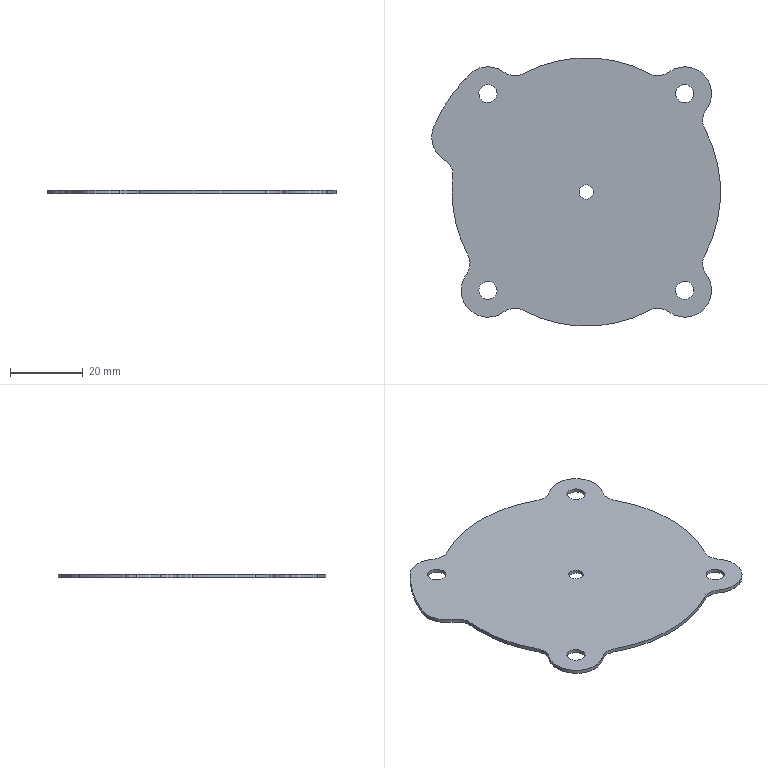Part | SolidWorks | features Cut 1, Extrusion 1 | 1 solid | 36 faces | box 79.627 x 74 x 1 mm | volume 4806 mm3 | cylinder 33 | plane 3 | commonest cylinder face diameters 10 x10 5 x8 14.784 x5 74 x5 4 x2 15 x2
STEP:
#1=CARTESIAN_POINT('',(2.,0.,1.));
#2=VERTEX_POINT('',#1);
#3=CARTESIAN_POINT('',(-2.,0.,1.));
#4=VERTEX_POINT('',#3);
#5=CARTESIAN_POINT('',(0.,0.,1.));
#6=DIRECTION('',(0.,0.,-1.));
#7=DIRECTION('',(-1.,0.,0.));
#8=AXIS2_PLACEMENT_3D('',#5,#6,#7);
#9=CIRCLE('',#8,2.);
#10=EDGE_CURVE('',#2,#4,#9,.T.);
#11=ORIENTED_EDGE('',*,*,#10,.F.);
#12=CARTESIAN_POINT('',(2.,0.,0.));
#13=VERTEX_POINT('',#12);
#14=CARTESIAN_POINT('',(2.,0.,1.));
#15=DIRECTION('',(0.,0.,-1.));
#16=VECTOR('',#15,1000.);
#17=LINE('',#14,#16);
#18=EDGE_CURVE('',#2,#13,#17,.T.);
#19=ORIENTED_EDGE('',*,*,#18,.T.);
#20=CARTESIAN_POINT('',(-2.,0.,0.));
#21=VERTEX_POINT('',#20);
#22=CARTESIAN_POINT('',(0.,0.,0.));
#23=DIRECTION('',(0.,0.,-1.));
#24=DIRECTION('',(-1.,0.,0.));
#25=AXIS2_PLACEMENT_3D('',#22,#23,#24);
#26=CIRCLE('',#25,2.);
#27=EDGE_CURVE('',#13,#21,#26,.T.);
#28=ORIENTED_EDGE('',*,*,#27,.T.);
#29=CARTESIAN_POINT('',(-2.,0.,1.));
#30=DIRECTION('',(0.,0.,-1.));
#31=VECTOR('',#30,1000.);
#32=LINE('',#29,#31);
#33=EDGE_CURVE('',#4,#21,#32,.T.);
#34=ORIENTED_EDGE('',*,*,#33,.F.);
#35=EDGE_LOOP('',(#11,#19,#28,#34));
#36=FACE_OUTER_BOUND('',#35,.T.);
#37=CARTESIAN_POINT('',(0.,0.,1.));
#38=DIRECTION('',(0.,0.,-1.));
#39=DIRECTION('',(-1.,0.,0.));
#40=AXIS2_PLACEMENT_3D('',#37,#38,#39);
#41=CYLINDRICAL_SURFACE('',#40,2.);
#42=ADVANCED_FACE('',(#36),#41,.F.);
#43=CARTESIAN_POINT('',(-29.633,27.133,1.));
#44=VERTEX_POINT('',#43);
#45=CARTESIAN_POINT('',(-24.633,27.133,1.));
#46=VERTEX_POINT('',#45);
#47=CARTESIAN_POINT('',(-29.633,27.133,1.));
#48=CARTESIAN_POINT('',(-29.633,26.098,1.));
#49=CARTESIAN_POINT('',(-28.901,25.366,1.));
#50=CARTESIAN_POINT('',(-28.169,24.633,1.));
#51=CARTESIAN_POINT('',(-27.133,24.633,1.));
#52=CARTESIAN_POINT('',(-26.098,24.633,1.));
#53=CARTESIAN_POINT('',(-25.366,25.366,1.));
#54=CARTESIAN_POINT('',(-24.633,26.098,1.));
#55=CARTESIAN_POINT('',(-24.633,27.133,1.));
#56=(BOUNDED_CURVE()B_SPLINE_CURVE(2,(#47,#48,#49,#50,#51,#52,#53,#54,#55),.UNSPECIFIED.,.F.,.T.)B_SPLINE_CURVE_WITH_KNOTS((3,2,2,2,3),(0.95,0.9583,0.9667,0.975,0.9833),.UNSPECIFIED.)CURVE()GEOMETRIC_REPRESENTATION_ITEM()RATIONAL_B_SPLINE_CURVE((1.,0.9239,1.,0.9239,1.,0.9239,1.,0.9239,1.))REPRESENTATION_ITEM(''));
#57=EDGE_CURVE('',#44,#46,#56,.T.);
#58=ORIENTED_EDGE('',*,*,#57,.T.);
#59=CARTESIAN_POINT('',(-24.633,27.133,0.));
#60=VERTEX_POINT('',#59);
#61=CARTESIAN_POINT('',(-24.633,27.133,1.));
#62=DIRECTION('',(0.,0.,-1.));
#63=VECTOR('',#62,1000.);
#64=LINE('',#61,#63);
#65=EDGE_CURVE('',#46,#60,#64,.T.);
#66=ORIENTED_EDGE('',*,*,#65,.T.);
#67=CARTESIAN_POINT('',(-29.633,27.133,0.));
#68=VERTEX_POINT('',#67);
#69=CARTESIAN_POINT('',(-29.633,27.133,0.));
#70=CARTESIAN_POINT('',(-29.633,26.098,0.));
#71=CARTESIAN_POINT('',(-28.901,25.366,0.));
#72=CARTESIAN_POINT('',(-28.169,24.633,0.));
#73=CARTESIAN_POINT('',(-27.133,24.633,0.));
#74=CARTESIAN_POINT('',(-26.098,24.633,0.));
#75=CARTESIAN_POINT('',(-25.366,25.366,0.));
#76=CARTESIAN_POINT('',(-24.633,26.098,0.));
#77=CARTESIAN_POINT('',(-24.633,27.133,0.));
#78=(BOUNDED_CURVE()B_SPLINE_CURVE(2,(#69,#70,#71,#72,#73,#74,#75,#76,#77),.UNSPECIFIED.,.F.,.F.)B_SPLINE_CURVE_WITH_KNOTS((3,2,2,2,3),(0.95,0.9583,0.9667,0.975,0.9833),.UNSPECIFIED.)CURVE()GEOMETRIC_REPRESENTATION_ITEM()RATIONAL_B_SPLINE_CURVE((1.,0.9239,1.,0.9239,1.,0.9239,1.,0.9239,1.))REPRESENTATION_ITEM(''));
#79=EDGE_CURVE('',#68,#60,#78,.T.);
#80=ORIENTED_EDGE('',*,*,#79,.F.);
#81=CARTESIAN_POINT('',(-29.633,27.133,1.));
#82=DIRECTION('',(0.,0.,-1.));
#83=VECTOR('',#82,1000.);
#84=LINE('',#81,#83);
#85=EDGE_CURVE('',#44,#68,#84,.T.);
#86=ORIENTED_EDGE('',*,*,#85,.F.);
#87=EDGE_LOOP('',(#58,#66,#80,#86));
#88=FACE_OUTER_BOUND('',#87,.T.);
#89=CARTESIAN_POINT('',(-27.133,27.133,1.));
#90=DIRECTION('',(0.,0.,-1.));
#91=DIRECTION('',(-1.,0.,0.));
#92=AXIS2_PLACEMENT_3D('',#89,#90,#91);
#93=CYLINDRICAL_SURFACE('',#92,2.5);
#94=ADVANCED_FACE('',(#88),#93,.F.);
#95=CARTESIAN_POINT('',(28.901,-28.901,1.));
#96=VERTEX_POINT('',#95);
#97=CARTESIAN_POINT('',(29.633,-27.133,1.));
#98=VERTEX_POINT('',#97);
#99=CARTESIAN_POINT('',(28.901,-28.901,1.));
#100=CARTESIAN_POINT('',(29.633,-28.169,1.));
#101=CARTESIAN_POINT('',(29.633,-27.133,1.));
#102=(BOUNDED_CURVE()B_SPLINE_CURVE(2,(#99,#100,#101),.UNSPECIFIED.,.F.,.F.)B_SPLINE_CURVE_WITH_KNOTS((3,3),(0.9417,0.95),.UNSPECIFIED.)CURVE()GEOMETRIC_REPRESENTATION_ITEM()RATIONAL_B_SPLINE_CURVE((1.,0.9239,1.))REPRESENTATION_ITEM(''));
#103=EDGE_CURVE('',#96,#98,#102,.T.);
#104=ORIENTED_EDGE('',*,*,#103,.T.);
#105=CARTESIAN_POINT('',(29.633,-27.133,0.));
#106=VERTEX_POINT('',#105);
#107=CARTESIAN_POINT('',(29.633,-27.133,1.));
#108=DIRECTION('',(0.,0.,-1.));
#109=VECTOR('',#108,1000.);
#110=LINE('',#107,#109);
#111=EDGE_CURVE('',#98,#106,#110,.T.);
#112=ORIENTED_EDGE('',*,*,#111,.T.);
#113=CARTESIAN_POINT('',(28.901,-28.901,0.));
#114=VERTEX_POINT('',#113);
#115=CARTESIAN_POINT('',(28.901,-28.901,0.));
#116=CARTESIAN_POINT('',(29.633,-28.169,0.));
#117=CARTESIAN_POINT('',(29.633,-27.133,0.));
#118=(BOUNDED_CURVE()B_SPLINE_CURVE(2,(#115,#116,#117),.UNSPECIFIED.,.F.,.T.)B_SPLINE_CURVE_WITH_KNOTS((3,3),(0.9417,0.95),.UNSPECIFIED.)CURVE()GEOMETRIC_REPRESENTATION_ITEM()RATIONAL_B_SPLINE_CURVE((1.,0.9239,1.))REPRESENTATION_ITEM(''));
#119=EDGE_CURVE('',#114,#106,#118,.T.);
#120=ORIENTED_EDGE('',*,*,#119,.F.);
#121=CARTESIAN_POINT('',(27.133,-29.633,0.));
#122=VERTEX_POINT('',#121);
#123=CARTESIAN_POINT('',(27.133,-27.133,0.));
#124=DIRECTION('',(0.,0.,1.));
#125=DIRECTION('',(1.,0.,0.));
#126=AXIS2_PLACEMENT_3D('',#123,#124,#125);
#127=CIRCLE('',#126,2.5);
#128=EDGE_CURVE('',#122,#114,#127,.T.);
#129=ORIENTED_EDGE('',*,*,#128,.F.);
#130=CARTESIAN_POINT('',(24.633,-27.133,0.));
#131=VERTEX_POINT('',#130);
#132=CARTESIAN_POINT('',(24.633,-27.133,0.));
#133=CARTESIAN_POINT('',(24.633,-28.169,0.));
#134=CARTESIAN_POINT('',(25.366,-28.901,0.));
#135=CARTESIAN_POINT('',(26.098,-29.633,0.));
#136=CARTESIAN_POINT('',(27.133,-29.633,0.));
#137=(BOUNDED_CURVE()B_SPLINE_CURVE(2,(#132,#133,#134,#135,#136),.UNSPECIFIED.,.F.,.T.)B_SPLINE_CURVE_WITH_KNOTS((3,2,3),(0.9833,0.9917,1.),.UNSPECIFIED.)CURVE()GEOMETRIC_REPRESENTATION_ITEM()RATIONAL_B_SPLINE_CURVE((1.,0.9239,1.,0.9239,1.))REPRESENTATION_ITEM(''));
#138=EDGE_CURVE('',#131,#122,#137,.T.);
#139=ORIENTED_EDGE('',*,*,#138,.F.);
#140=CARTESIAN_POINT('',(24.633,-27.133,1.));
#141=VERTEX_POINT('',#140);
#142=CARTESIAN_POINT('',(24.633,-27.133,1.));
#143=DIRECTION('',(0.,0.,-1.));
#144=VECTOR('',#143,1000.);
#145=LINE('',#142,#144);
#146=EDGE_CURVE('',#141,#131,#145,.T.);
#147=ORIENTED_EDGE('',*,*,#146,.F.);
#148=CARTESIAN_POINT('',(27.133,-29.633,1.));
#149=VERTEX_POINT('',#148);
#150=CARTESIAN_POINT('',(24.633,-27.133,1.));
#151=CARTESIAN_POINT('',(24.633,-28.169,1.));
#152=CARTESIAN_POINT('',(25.366,-28.901,1.));
#153=CARTESIAN_POINT('',(26.098,-29.633,1.));
#154=CARTESIAN_POINT('',(27.133,-29.633,1.));
#155=(BOUNDED_CURVE()B_SPLINE_CURVE(2,(#150,#151,#152,#153,#154),.UNSPECIFIED.,.F.,.F.)B_SPLINE_CURVE_WITH_KNOTS((3,2,3),(0.9833,0.9917,1.),.UNSPECIFIED.)CURVE()GEOMETRIC_REPRESENTATION_ITEM()RATIONAL_B_SPLINE_CURVE((1.,0.9239,1.,0.9239,1.))REPRESENTATION_ITEM(''));
#156=EDGE_CURVE('',#141,#149,#155,.T.);
#157=ORIENTED_EDGE('',*,*,#156,.T.);
#158=CARTESIAN_POINT('',(27.133,-27.133,1.));
#159=DIRECTION('',(0.,0.,1.));
#160=DIRECTION('',(1.,0.,0.));
#161=AXIS2_PLACEMENT_3D('',#158,#159,#160);
#162=CIRCLE('',#161,2.5);
#163=EDGE_CURVE('',#149,#96,#162,.T.);
#164=ORIENTED_EDGE('',*,*,#163,.T.);
#165=EDGE_LOOP('',(#104,#112,#120,#129,#139,#147,#157,#164));
#166=FACE_OUTER_BOUND('',#165,.T.);
#167=CARTESIAN_POINT('',(27.133,-27.133,1.));
#168=DIRECTION('',(0.,0.,-1.));
#169=DIRECTION('',(-1.,0.,0.));
#170=AXIS2_PLACEMENT_3D('',#167,#168,#169);
#171=CYLINDRICAL_SURFACE('',#170,2.5);
#172=ADVANCED_FACE('',(#166),#171,.F.);
#173=CARTESIAN_POINT('',(24.633,27.133,1.));
#174=VERTEX_POINT('',#173);
#175=CARTESIAN_POINT('',(29.633,27.133,1.));
#176=VERTEX_POINT('',#175);
#177=CARTESIAN_POINT('',(27.133,27.133,1.));
#178=DIRECTION('',(0.,0.,1.));
#179=DIRECTION('',(1.,0.,0.));
#180=AXIS2_PLACEMENT_3D('',#177,#178,#179);
#181=CIRCLE('',#180,2.5);
#182=EDGE_CURVE('',#174,#176,#181,.T.);
#183=ORIENTED_EDGE('',*,*,#182,.T.);
#184=CARTESIAN_POINT('',(29.633,27.133,0.));
#185=VERTEX_POINT('',#184);
#186=CARTESIAN_POINT('',(29.633,27.133,1.));
#187=DIRECTION('',(0.,0.,-1.));
#188=VECTOR('',#187,1000.);
#189=LINE('',#186,#188);
#190=EDGE_CURVE('',#176,#185,#189,.T.);
#191=ORIENTED_EDGE('',*,*,#190,.T.);
#192=CARTESIAN_POINT('',(24.633,27.133,0.));
#193=VERTEX_POINT('',#192);
#194=CARTESIAN_POINT('',(27.133,27.133,0.));
#195=DIRECTION('',(0.,0.,1.));
#196=DIRECTION('',(1.,0.,0.));
#197=AXIS2_PLACEMENT_3D('',#194,#195,#196);
#198=CIRCLE('',#197,2.5);
#199=EDGE_CURVE('',#193,#185,#198,.T.);
#200=ORIENTED_EDGE('',*,*,#199,.F.);
#201=CARTESIAN_POINT('',(24.633,27.133,1.));
#202=DIRECTION('',(0.,0.,-1.));
#203=VECTOR('',#202,1000.);
#204=LINE('',#201,#203);
#205=EDGE_CURVE('',#174,#193,#204,.T.);
#206=ORIENTED_EDGE('',*,*,#205,.F.);
#207=EDGE_LOOP('',(#183,#191,#200,#206));
#208=FACE_OUTER_BOUND('',#207,.T.);
#209=CARTESIAN_POINT('',(27.133,27.133,1.));
#210=DIRECTION('',(0.,0.,-1.));
#211=DIRECTION('',(-1.,0.,0.));
#212=AXIS2_PLACEMENT_3D('',#209,#210,#211);
#213=CYLINDRICAL_SURFACE('',#212,2.5);
#214=ADVANCED_FACE('',(#208),#213,.F.);
#215=CARTESIAN_POINT('',(-28.901,-28.901,1.));
#216=VERTEX_POINT('',#215);
#217=CARTESIAN_POINT('',(-24.633,-27.133,1.));
#218=VERTEX_POINT('',#217);
#219=CARTESIAN_POINT('',(-28.901,-28.901,1.));
#220=CARTESIAN_POINT('',(-28.169,-29.633,1.));
#221=CARTESIAN_POINT('',(-27.133,-29.633,1.));
#222=CARTESIAN_POINT('',(-26.098,-29.633,1.));
#223=CARTESIAN_POINT('',(-25.366,-28.901,1.));
#224=CARTESIAN_POINT('',(-24.633,-28.169,1.));
#225=CARTESIAN_POINT('',(-24.633,-27.133,1.));
#226=(BOUNDED_CURVE()B_SPLINE_CURVE(2,(#219,#220,#221,#222,#223,#224,#225),.UNSPECIFIED.,.F.,.T.)B_SPLINE_CURVE_WITH_KNOTS((3,2,2,3),(0.9417,0.95,0.9583,0.9667),.UNSPECIFIED.)CURVE()GEOMETRIC_REPRESENTATION_ITEM()RATIONAL_B_SPLINE_CURVE((1.,0.9239,1.,0.9239,1.,0.9239,1.))REPRESENTATION_ITEM(''));
#227=EDGE_CURVE('',#216,#218,#226,.T.);
#228=ORIENTED_EDGE('',*,*,#227,.T.);
#229=CARTESIAN_POINT('',(-24.633,-27.133,0.));
#230=VERTEX_POINT('',#229);
#231=CARTESIAN_POINT('',(-24.633,-27.133,1.));
#232=DIRECTION('',(0.,0.,-1.));
#233=VECTOR('',#232,1000.);
#234=LINE('',#231,#233);
#235=EDGE_CURVE('',#218,#230,#234,.T.);
#236=ORIENTED_EDGE('',*,*,#235,.T.);
#237=CARTESIAN_POINT('',(-28.901,-28.901,0.));
#238=VERTEX_POINT('',#237);
#239=CARTESIAN_POINT('',(-28.901,-28.901,0.));
#240=CARTESIAN_POINT('',(-28.169,-29.633,0.));
#241=CARTESIAN_POINT('',(-27.133,-29.633,0.));
#242=CARTESIAN_POINT('',(-26.098,-29.633,0.));
#243=CARTESIAN_POINT('',(-25.366,-28.901,0.));
#244=CARTESIAN_POINT('',(-24.633,-28.169,0.));
#245=CARTESIAN_POINT('',(-24.633,-27.133,0.));
#246=(BOUNDED_CURVE()B_SPLINE_CURVE(2,(#239,#240,#241,#242,#243,#244,#245),.UNSPECIFIED.,.F.,.T.)B_SPLINE_CURVE_WITH_KNOTS((3,2,2,3),(0.9417,0.95,0.9583,0.9667),.UNSPECIFIED.)CURVE()GEOMETRIC_REPRESENTATION_ITEM()RATIONAL_B_SPLINE_CURVE((1.,0.9239,1.,0.9239,1.,0.9239,1.))REPRESENTATION_ITEM(''));
#247=EDGE_CURVE('',#238,#230,#246,.T.);
#248=ORIENTED_EDGE('',*,*,#247,.F.);
#249=CARTESIAN_POINT('',(-29.633,-27.133,0.));
#250=VERTEX_POINT('',#249);
#251=CARTESIAN_POINT('',(-27.133,-27.133,0.));
#252=DIRECTION('',(0.,0.,1.));
#253=DIRECTION('',(1.,0.,0.));
#254=AXIS2_PLACEMENT_3D('',#251,#252,#253);
#255=CIRCLE('',#254,2.5);
#256=EDGE_CURVE('',#250,#238,#255,.T.);
#257=ORIENTED_EDGE('',*,*,#256,.F.);
#258=CARTESIAN_POINT('',(-29.633,-27.133,1.));
#259=VERTEX_POINT('',#258);
#260=CARTESIAN_POINT('',(-29.633,-27.133,1.));
#261=DIRECTION('',(0.,0.,-1.));
#262=VECTOR('',#261,1000.);
#263=LINE('',#260,#262);
#264=EDGE_CURVE('',#259,#250,#263,.T.);
#265=ORIENTED_EDGE('',*,*,#264,.F.);
#266=CARTESIAN_POINT('',(-27.133,-27.133,1.));
#267=DIRECTION('',(0.,0.,1.));
#268=DIRECTION('',(1.,0.,0.));
#269=AXIS2_PLACEMENT_3D('',#266,#267,#268);
#270=CIRCLE('',#269,2.5);
#271=EDGE_CURVE('',#259,#216,#270,.T.);
#272=ORIENTED_EDGE('',*,*,#271,.T.);
#273=EDGE_LOOP('',(#228,#236,#248,#257,#265,#272));
#274=FACE_OUTER_BOUND('',#273,.T.);
#275=CARTESIAN_POINT('',(-27.133,-27.133,1.));
#276=DIRECTION('',(0.,0.,-1.));
#277=DIRECTION('',(-1.,0.,0.));
#278=AXIS2_PLACEMENT_3D('',#275,#276,#277);
#279=CYLINDRICAL_SURFACE('',#278,2.5);
#280=ADVANCED_FACE('',(#274),#279,.F.);
#281=CARTESIAN_POINT('',(32.075,19.735,1.));
#282=VERTEX_POINT('',#281);
#283=CARTESIAN_POINT('',(33.064,22.72,1.));
#284=VERTEX_POINT('',#283);
#285=CARTESIAN_POINT('',(37.075,19.735,1.));
#286=DIRECTION('',(0.,0.,-1.));
#287=DIRECTION('',(1.,0.,0.));
#288=AXIS2_PLACEMENT_3D('',#285,#286,#287);
#289=CIRCLE('',#288,5.);
#290=EDGE_CURVE('',#282,#284,#289,.T.);
#291=ORIENTED_EDGE('',*,*,#290,.F.);
#292=CARTESIAN_POINT('',(32.075,19.735,0.));
#293=VERTEX_POINT('',#292);
#294=CARTESIAN_POINT('',(32.075,19.735,1.));
#295=DIRECTION('',(0.,0.,-1.));
#296=VECTOR('',#295,1000.);
#297=LINE('',#294,#296);
#298=EDGE_CURVE('',#282,#293,#297,.T.);
#299=ORIENTED_EDGE('',*,*,#298,.T.);
#300=CARTESIAN_POINT('',(33.064,22.72,0.));
#301=VERTEX_POINT('',#300);
#302=CARTESIAN_POINT('',(37.075,19.735,0.));
#303=DIRECTION('',(0.,0.,-1.));
#304=DIRECTION('',(1.,0.,0.));
#305=AXIS2_PLACEMENT_3D('',#302,#303,#304);
#306=CIRCLE('',#305,5.);
#307=EDGE_CURVE('',#293,#301,#306,.T.);
#308=ORIENTED_EDGE('',*,*,#307,.T.);
#309=CARTESIAN_POINT('',(33.064,22.72,1.));
#310=DIRECTION('',(0.,0.,-1.));
#311=VECTOR('',#310,1000.);
#312=LINE('',#309,#311);
#313=EDGE_CURVE('',#284,#301,#312,.T.);
#314=ORIENTED_EDGE('',*,*,#313,.F.);
#315=EDGE_LOOP('',(#291,#299,#308,#314));
#316=FACE_OUTER_BOUND('',#315,.T.);
#317=CARTESIAN_POINT('',(37.075,19.735,1.));
#318=DIRECTION('',(0.,0.,-1.));
#319=DIRECTION('',(-1.,0.,0.));
#320=AXIS2_PLACEMENT_3D('',#317,#318,#319);
#321=CYLINDRICAL_SURFACE('',#320,5.);
#322=ADVANCED_FACE('',(#316),#321,.F.);
#323=CARTESIAN_POINT('',(32.075,-19.735,1.));
#324=VERTEX_POINT('',#323);
#325=CARTESIAN_POINT('',(32.661,-17.386,1.));
#326=VERTEX_POINT('',#325);
#327=CARTESIAN_POINT('',(37.075,-19.735,1.));
#328=DIRECTION('',(0.,0.,-1.));
#329=DIRECTION('',(1.,0.,0.));
#330=AXIS2_PLACEMENT_3D('',#327,#328,#329);
#331=CIRCLE('',#330,5.);
#332=EDGE_CURVE('',#324,#326,#331,.T.);
#333=ORIENTED_EDGE('',*,*,#332,.F.);
#334=CARTESIAN_POINT('',(32.075,-19.735,0.));
#335=VERTEX_POINT('',#334);
#336=CARTESIAN_POINT('',(32.075,-19.735,1.));
#337=DIRECTION('',(0.,0.,-1.));
#338=VECTOR('',#337,1000.);
#339=LINE('',#336,#338);
#340=EDGE_CURVE('',#324,#335,#339,.T.);
#341=ORIENTED_EDGE('',*,*,#340,.T.);
#342=CARTESIAN_POINT('',(32.661,-17.386,0.));
#343=VERTEX_POINT('',#342);
#344=CARTESIAN_POINT('',(37.075,-19.735,0.));
#345=DIRECTION('',(0.,0.,-1.));
#346=DIRECTION('',(1.,0.,0.));
#347=AXIS2_PLACEMENT_3D('',#344,#345,#346);
#348=CIRCLE('',#347,5.);
#349=EDGE_CURVE('',#335,#343,#348,.T.);
#350=ORIENTED_EDGE('',*,*,#349,.T.);
#351=CARTESIAN_POINT('',(32.661,-17.386,1.));
#352=DIRECTION('',(0.,0.,-1.));
#353=VECTOR('',#352,1000.);
#354=LINE('',#351,#353);
#355=EDGE_CURVE('',#326,#343,#354,.T.);
#356=ORIENTED_EDGE('',*,*,#355,.F.);
#357=EDGE_LOOP('',(#333,#341,#350,#356));
#358=FACE_OUTER_BOUND('',#357,.T.);
#359=CARTESIAN_POINT('',(37.075,-19.735,1.));
#360=DIRECTION('',(0.,0.,-1.));
#361=DIRECTION('',(-1.,0.,0.));
#362=AXIS2_PLACEMENT_3D('',#359,#360,#361);
#363=CYLINDRICAL_SURFACE('',#362,5.);
#364=ADVANCED_FACE('',(#358),#363,.F.);
#365=CARTESIAN_POINT('',(-34.526,-27.133,1.));
#366=VERTEX_POINT('',#365);
#367=CARTESIAN_POINT('',(-22.72,-33.064,1.));
#368=VERTEX_POINT('',#367);
#369=CARTESIAN_POINT('',(-27.133,-27.133,1.));
#370=DIRECTION('',(0.,0.,1.));
#371=DIRECTION('',(1.,0.,0.));
#372=AXIS2_PLACEMENT_3D('',#369,#370,#371);
#373=CIRCLE('',#372,7.392);
#374=EDGE_CURVE('',#366,#368,#373,.T.);
#375=ORIENTED_EDGE('',*,*,#374,.F.);
#376=CARTESIAN_POINT('',(-34.526,-27.133,0.));
#377=VERTEX_POINT('',#376);
#378=CARTESIAN_POINT('',(-34.526,-27.133,1.));
#379=DIRECTION('',(0.,0.,-1.));
#380=VECTOR('',#379,1000.);
#381=LINE('',#378,#380);
#382=EDGE_CURVE('',#366,#377,#381,.T.);
#383=ORIENTED_EDGE('',*,*,#382,.T.);
#384=CARTESIAN_POINT('',(-22.72,-33.064,0.));
#385=VERTEX_POINT('',#384);
#386=CARTESIAN_POINT('',(-27.133,-27.133,0.));
#387=DIRECTION('',(0.,0.,1.));
#388=DIRECTION('',(1.,0.,0.));
#389=AXIS2_PLACEMENT_3D('',#386,#387,#388);
#390=CIRCLE('',#389,7.392);
#391=EDGE_CURVE('',#377,#385,#390,.T.);
#392=ORIENTED_EDGE('',*,*,#391,.T.);
#393=CARTESIAN_POINT('',(-22.72,-33.064,1.));
#394=DIRECTION('',(0.,0.,-1.));
#395=VECTOR('',#394,1000.);
#396=LINE('',#393,#395);
#397=EDGE_CURVE('',#368,#385,#396,.T.);
#398=ORIENTED_EDGE('',*,*,#397,.F.);
#399=EDGE_LOOP('',(#375,#383,#392,#398));
#400=FACE_OUTER_BOUND('',#399,.T.);
#401=CARTESIAN_POINT('',(-27.133,-27.133,1.));
#402=DIRECTION('',(0.,0.,-1.));
#403=DIRECTION('',(-1.,0.,0.));
#404=AXIS2_PLACEMENT_3D('',#401,#402,#403);
#405=CYLINDRICAL_SURFACE('',#404,7.392);
#406=ADVANCED_FACE('',(#400),#405,.T.);
#407=CARTESIAN_POINT('',(-37.,0.,1.));
#408=VERTEX_POINT('',#407);
#409=CARTESIAN_POINT('',(-32.661,-17.386,1.));
#410=VERTEX_POINT('',#409);
#411=CARTESIAN_POINT('',(0.,0.,1.));
#412=DIRECTION('',(0.,0.,1.));
#413=DIRECTION('',(1.,0.,0.));
#414=AXIS2_PLACEMENT_3D('',#411,#412,#413);
#415=CIRCLE('',#414,37.);
#416=EDGE_CURVE('',#408,#410,#415,.T.);
#417=ORIENTED_EDGE('',*,*,#416,.F.);
#418=CARTESIAN_POINT('',(-37.,0.,0.));
#419=VERTEX_POINT('',#418);
#420=CARTESIAN_POINT('',(-37.,0.,1.));
#421=DIRECTION('',(0.,0.,-1.));
#422=VECTOR('',#421,1000.);
#423=LINE('',#420,#422);
#424=EDGE_CURVE('',#408,#419,#423,.T.);
#425=ORIENTED_EDGE('',*,*,#424,.T.);
#426=CARTESIAN_POINT('',(-32.661,-17.386,0.));
#427=VERTEX_POINT('',#426);
#428=CARTESIAN_POINT('',(0.,0.,0.));
#429=DIRECTION('',(0.,0.,1.));
#430=DIRECTION('',(1.,0.,0.));
#431=AXIS2_PLACEMENT_3D('',#428,#429,#430);
#432=CIRCLE('',#431,37.);
#433=EDGE_CURVE('',#419,#427,#432,.T.);
#434=ORIENTED_EDGE('',*,*,#433,.T.);
#435=CARTESIAN_POINT('',(-32.661,-17.386,1.));
#436=DIRECTION('',(0.,0.,-1.));
#437=VECTOR('',#436,1000.);
#438=LINE('',#435,#437);
#439=EDGE_CURVE('',#410,#427,#438,.T.);
#440=ORIENTED_EDGE('',*,*,#439,.F.);
#441=EDGE_LOOP('',(#417,#425,#434,#440));
#442=FACE_OUTER_BOUND('',#441,.T.);
#443=CARTESIAN_POINT('',(0.,0.,1.));
#444=DIRECTION('',(0.,0.,-1.));
#445=DIRECTION('',(-1.,0.,0.));
#446=AXIS2_PLACEMENT_3D('',#443,#444,#445);
#447=CYLINDRICAL_SURFACE('',#446,37.);
#448=ADVANCED_FACE('',(#442),#447,.T.);
#449=CARTESIAN_POINT('',(-42.627,15.175,1.));
#450=VERTEX_POINT('',#449);
#451=CARTESIAN_POINT('',(-39.101,8.815,1.));
#452=VERTEX_POINT('',#451);
#453=CARTESIAN_POINT('',(-35.127,15.175,1.));
#454=DIRECTION('',(0.,0.,1.));
#455=DIRECTION('',(1.,0.,0.));
#456=AXIS2_PLACEMENT_3D('',#453,#454,#455);
#457=CIRCLE('',#456,7.5);
#458=EDGE_CURVE('',#450,#452,#457,.T.);
#459=ORIENTED_EDGE('',*,*,#458,.F.);
#460=CARTESIAN_POINT('',(-42.627,15.175,0.));
#461=VERTEX_POINT('',#460);
#462=CARTESIAN_POINT('',(-42.627,15.175,1.));
#463=DIRECTION('',(0.,0.,-1.));
#464=VECTOR('',#463,1000.);
#465=LINE('',#462,#464);
#466=EDGE_CURVE('',#450,#461,#465,.T.);
#467=ORIENTED_EDGE('',*,*,#466,.T.);
#468=CARTESIAN_POINT('',(-39.101,8.815,0.));
#469=VERTEX_POINT('',#468);
#470=CARTESIAN_POINT('',(-35.127,15.175,0.));
#471=DIRECTION('',(0.,0.,1.));
#472=DIRECTION('',(1.,0.,0.));
#473=AXIS2_PLACEMENT_3D('',#470,#471,#472);
#474=CIRCLE('',#473,7.5);
#475=EDGE_CURVE('',#461,#469,#474,.T.);
#476=ORIENTED_EDGE('',*,*,#475,.T.);
#477=CARTESIAN_POINT('',(-39.101,8.815,1.));
#478=DIRECTION('',(0.,0.,-1.));
#479=VECTOR('',#478,1000.);
#480=LINE('',#477,#479);
#481=EDGE_CURVE('',#452,#469,#480,.T.);
#482=ORIENTED_EDGE('',*,*,#481,.F.);
#483=EDGE_LOOP('',(#459,#467,#476,#482));
#484=FACE_OUTER_BOUND('',#483,.T.);
#485=CARTESIAN_POINT('',(-35.127,15.175,1.));
#486=DIRECTION('',(0.,0.,-1.));
#487=DIRECTION('',(-1.,0.,0.));
#488=AXIS2_PLACEMENT_3D('',#485,#486,#487);
#489=CYLINDRICAL_SURFACE('',#488,7.5);
#490=ADVANCED_FACE('',(#484),#489,.T.);
#491=CARTESIAN_POINT('',(0.,0.,1.));
#492=DIRECTION('',(0.,0.,-1.));
#493=DIRECTION('',(-1.,0.,0.));
#494=AXIS2_PLACEMENT_3D('',#491,#492,#493);
#495=CIRCLE('',#494,2.);
#496=EDGE_CURVE('',#4,#2,#495,.T.);
#497=ORIENTED_EDGE('',*,*,#496,.T.);
#498=ORIENTED_EDGE('',*,*,#10,.T.);
#499=EDGE_LOOP('',(#497,#498));
#500=FACE_BOUND('',#499,.T.);
#501=ORIENTED_EDGE('',*,*,#227,.F.);
#502=ORIENTED_EDGE('',*,*,#271,.F.);
#503=CARTESIAN_POINT('',(-24.633,-27.133,1.));
#504=CARTESIAN_POINT('',(-24.633,-26.098,1.));
#505=CARTESIAN_POINT('',(-25.366,-25.366,1.));
#506=CARTESIAN_POINT('',(-26.098,-24.633,1.));
#507=CARTESIAN_POINT('',(-27.133,-24.633,1.));
#508=CARTESIAN_POINT('',(-28.169,-24.633,1.));
#509=CARTESIAN_POINT('',(-28.901,-25.366,1.));
#510=CARTESIAN_POINT('',(-29.633,-26.098,1.));
#511=CARTESIAN_POINT('',(-29.633,-27.133,1.));
#512=(BOUNDED_CURVE()B_SPLINE_CURVE(2,(#503,#504,#505,#506,#507,#508,#509,#510,#511),.UNSPECIFIED.,.F.,.F.)B_SPLINE_CURVE_WITH_KNOTS((3,2,2,2,3),(0.9667,0.975,0.9833,0.9917,1.),.UNSPECIFIED.)CURVE()GEOMETRIC_REPRESENTATION_ITEM()RATIONAL_B_SPLINE_CURVE((1.,0.9239,1.,0.9239,1.,0.9239,1.,0.9239,1.))REPRESENTATION_ITEM(''));
#513=EDGE_CURVE('',#218,#259,#512,.T.);
#514=ORIENTED_EDGE('',*,*,#513,.F.);
#515=EDGE_LOOP('',(#501,#502,#514));
#516=FACE_BOUND('',#515,.T.);
#517=CARTESIAN_POINT('',(-33.455,31.228,1.));
#518=VERTEX_POINT('',#517);
#519=CARTESIAN_POINT('',(-42.012,18.15,1.));
#520=VERTEX_POINT('',#519);
#521=CARTESIAN_POINT('',(0.,0.,1.));
#522=DIRECTION('',(0.,0.,1.));
#523=DIRECTION('',(1.,0.,0.));
#524=AXIS2_PLACEMENT_3D('',#521,#522,#523);
#525=CIRCLE('',#524,45.765);
#526=EDGE_CURVE('',#518,#520,#525,.T.);
#527=ORIENTED_EDGE('',*,*,#526,.T.);
#528=CARTESIAN_POINT('',(-35.127,15.175,1.));
#529=DIRECTION('',(0.,0.,1.));
#530=DIRECTION('',(1.,0.,0.));
#531=AXIS2_PLACEMENT_3D('',#528,#529,#530);
#532=CIRCLE('',#531,7.5);
#533=EDGE_CURVE('',#520,#450,#532,.T.);
#534=ORIENTED_EDGE('',*,*,#533,.T.);
#535=ORIENTED_EDGE('',*,*,#458,.T.);
#536=CARTESIAN_POINT('',(-36.78,4.03,1.));
#537=VERTEX_POINT('',#536);
#538=CARTESIAN_POINT('',(-41.75,4.574,1.));
#539=DIRECTION('',(0.,0.,-1.));
#540=DIRECTION('',(1.,0.,0.));
#541=AXIS2_PLACEMENT_3D('',#538,#539,#540);
#542=CIRCLE('',#541,5.);
#543=EDGE_CURVE('',#452,#537,#542,.T.);
#544=ORIENTED_EDGE('',*,*,#543,.T.);
#545=CARTESIAN_POINT('',(0.,0.,1.));
#546=DIRECTION('',(0.,0.,1.));
#547=DIRECTION('',(1.,0.,0.));
#548=AXIS2_PLACEMENT_3D('',#545,#546,#547);
#549=CIRCLE('',#548,37.);
#550=EDGE_CURVE('',#537,#408,#549,.T.);
#551=ORIENTED_EDGE('',*,*,#550,.T.);
#552=ORIENTED_EDGE('',*,*,#416,.T.);
#553=CARTESIAN_POINT('',(-33.064,-22.72,1.));
#554=VERTEX_POINT('',#553);
#555=CARTESIAN_POINT('',(-37.075,-19.735,1.));
#556=DIRECTION('',(0.,0.,-1.));
#557=DIRECTION('',(1.,0.,0.));
#558=AXIS2_PLACEMENT_3D('',#555,#556,#557);
#559=CIRCLE('',#558,5.);
#560=EDGE_CURVE('',#410,#554,#559,.T.);
#561=ORIENTED_EDGE('',*,*,#560,.T.);
#562=CARTESIAN_POINT('',(-27.133,-27.133,1.));
#563=DIRECTION('',(0.,0.,1.));
#564=DIRECTION('',(1.,0.,0.));
#565=AXIS2_PLACEMENT_3D('',#562,#563,#564);
#566=CIRCLE('',#565,7.392);
#567=EDGE_CURVE('',#554,#366,#566,.T.);
#568=ORIENTED_EDGE('',*,*,#567,.T.);
#569=ORIENTED_EDGE('',*,*,#374,.T.);
#570=CARTESIAN_POINT('',(-17.386,-32.661,1.));
#571=VERTEX_POINT('',#570);
#572=CARTESIAN_POINT('',(-19.735,-37.075,1.));
#573=DIRECTION('',(0.,0.,-1.));
#574=DIRECTION('',(1.,0.,0.));
#575=AXIS2_PLACEMENT_3D('',#572,#573,#574);
#576=CIRCLE('',#575,5.);
#577=EDGE_CURVE('',#368,#571,#576,.T.);
#578=ORIENTED_EDGE('',*,*,#577,.T.);
#579=CARTESIAN_POINT('',(17.386,-32.661,1.));
#580=VERTEX_POINT('',#579);
#581=CARTESIAN_POINT('',(0.,0.,1.));
#582=DIRECTION('',(0.,0.,1.));
#583=DIRECTION('',(1.,0.,0.));
#584=AXIS2_PLACEMENT_3D('',#581,#582,#583);
#585=CIRCLE('',#584,37.);
#586=EDGE_CURVE('',#571,#580,#585,.T.);
#587=ORIENTED_EDGE('',*,*,#586,.T.);
#588=CARTESIAN_POINT('',(22.72,-33.064,1.));
#589=VERTEX_POINT('',#588);
#590=CARTESIAN_POINT('',(19.735,-37.075,1.));
#591=DIRECTION('',(0.,0.,-1.));
#592=DIRECTION('',(1.,0.,0.));
#593=AXIS2_PLACEMENT_3D('',#590,#591,#592);
#594=CIRCLE('',#593,5.);
#595=EDGE_CURVE('',#580,#589,#594,.T.);
#596=ORIENTED_EDGE('',*,*,#595,.T.);
#597=CARTESIAN_POINT('',(33.064,-22.72,1.));
#598=VERTEX_POINT('',#597);
#599=CARTESIAN_POINT('',(27.133,-27.133,1.));
#600=DIRECTION('',(0.,0.,1.));
#601=DIRECTION('',(1.,0.,0.));
#602=AXIS2_PLACEMENT_3D('',#599,#600,#601);
#603=CIRCLE('',#602,7.392);
#604=EDGE_CURVE('',#589,#598,#603,.T.);
#605=ORIENTED_EDGE('',*,*,#604,.T.);
#606=CARTESIAN_POINT('',(37.075,-19.735,1.));
#607=DIRECTION('',(0.,0.,-1.));
#608=DIRECTION('',(1.,0.,0.));
#609=AXIS2_PLACEMENT_3D('',#606,#607,#608);
#610=CIRCLE('',#609,5.);
#611=EDGE_CURVE('',#598,#324,#610,.T.);
#612=ORIENTED_EDGE('',*,*,#611,.T.);
#613=ORIENTED_EDGE('',*,*,#332,.T.);
#614=CARTESIAN_POINT('',(32.661,17.386,1.));
#615=VERTEX_POINT('',#614);
#616=CARTESIAN_POINT('',(0.,0.,1.));
#617=DIRECTION('',(0.,0.,1.));
#618=DIRECTION('',(1.,0.,0.));
#619=AXIS2_PLACEMENT_3D('',#616,#617,#618);
#620=CIRCLE('',#619,37.);
#621=EDGE_CURVE('',#326,#615,#620,.T.);
#622=ORIENTED_EDGE('',*,*,#621,.T.);
#623=CARTESIAN_POINT('',(37.075,19.735,1.));
#624=DIRECTION('',(0.,0.,-1.));
#625=DIRECTION('',(1.,0.,0.));
#626=AXIS2_PLACEMENT_3D('',#623,#624,#625);
#627=CIRCLE('',#626,5.);
#628=EDGE_CURVE('',#615,#282,#627,.T.);
#629=ORIENTED_EDGE('',*,*,#628,.T.);
#630=ORIENTED_EDGE('',*,*,#290,.T.);
#631=CARTESIAN_POINT('',(22.72,33.064,1.));
#632=VERTEX_POINT('',#631);
#633=CARTESIAN_POINT('',(27.133,27.133,1.));
#634=DIRECTION('',(0.,0.,1.));
#635=DIRECTION('',(1.,0.,0.));
#636=AXIS2_PLACEMENT_3D('',#633,#634,#635);
#637=CIRCLE('',#636,7.392);
#638=EDGE_CURVE('',#284,#632,#637,.T.);
#639=ORIENTED_EDGE('',*,*,#638,.T.);
#640=CARTESIAN_POINT('',(17.386,32.661,1.));
#641=VERTEX_POINT('',#640);
#642=CARTESIAN_POINT('',(19.735,37.075,1.));
#643=DIRECTION('',(0.,0.,-1.));
#644=DIRECTION('',(1.,0.,0.));
#645=AXIS2_PLACEMENT_3D('',#642,#643,#644);
#646=CIRCLE('',#645,5.);
#647=EDGE_CURVE('',#632,#641,#646,.T.);
#648=ORIENTED_EDGE('',*,*,#647,.T.);
#649=CARTESIAN_POINT('',(-17.386,32.661,1.));
#650=VERTEX_POINT('',#649);
#651=CARTESIAN_POINT('',(0.,0.,1.));
#652=DIRECTION('',(0.,0.,1.));
#653=DIRECTION('',(1.,0.,0.));
#654=AXIS2_PLACEMENT_3D('',#651,#652,#653);
#655=CIRCLE('',#654,37.);
#656=EDGE_CURVE('',#641,#650,#655,.T.);
#657=ORIENTED_EDGE('',*,*,#656,.T.);
#658=CARTESIAN_POINT('',(-22.72,33.064,1.));
#659=VERTEX_POINT('',#658);
#660=CARTESIAN_POINT('',(-19.735,37.075,1.));
#661=DIRECTION('',(0.,0.,-1.));
#662=DIRECTION('',(1.,0.,0.));
#663=AXIS2_PLACEMENT_3D('',#660,#661,#662);
#664=CIRCLE('',#663,5.);
#665=EDGE_CURVE('',#650,#659,#664,.T.);
#666=ORIENTED_EDGE('',*,*,#665,.T.);
#667=CARTESIAN_POINT('',(-33.388,31.073,1.));
#668=VERTEX_POINT('',#667);
#669=CARTESIAN_POINT('',(-27.133,27.133,1.));
#670=DIRECTION('',(0.,0.,1.));
#671=DIRECTION('',(1.,0.,0.));
#672=AXIS2_PLACEMENT_3D('',#669,#670,#671);
#673=CIRCLE('',#672,7.392);
#674=EDGE_CURVE('',#659,#668,#673,.T.);
#675=ORIENTED_EDGE('',*,*,#674,.T.);
#676=CARTESIAN_POINT('',(-33.388,31.073,1.));
#677=DIRECTION('',(-0.3968,0.9179,0.));
#678=VECTOR('',#677,1000.);
#679=LINE('',#676,#678);
#680=EDGE_CURVE('',#668,#518,#679,.T.);
#681=ORIENTED_EDGE('',*,*,#680,.T.);
#682=EDGE_LOOP('',(#527,#534,#535,#544,#551,#552,#561,#568,#569,#578,#587,#596,#605,#612,#613,#622,#629,#630,#639,#648,#657,#666,#675,#681));
#683=FACE_OUTER_BOUND('',#682,.T.);
#684=ORIENTED_EDGE('',*,*,#182,.F.);
#685=CARTESIAN_POINT('',(27.133,27.133,1.));
#686=DIRECTION('',(0.,0.,1.));
#687=DIRECTION('',(1.,0.,0.));
#688=AXIS2_PLACEMENT_3D('',#685,#686,#687);
#689=CIRCLE('',#688,2.5);
#690=EDGE_CURVE('',#176,#174,#689,.T.);
#691=ORIENTED_EDGE('',*,*,#690,.F.);
#692=EDGE_LOOP('',(#684,#691));
#693=FACE_BOUND('',#692,.T.);
#694=ORIENTED_EDGE('',*,*,#103,.F.);
#695=ORIENTED_EDGE('',*,*,#163,.F.);
#696=ORIENTED_EDGE('',*,*,#156,.F.);
#697=CARTESIAN_POINT('',(29.633,-27.133,1.));
#698=CARTESIAN_POINT('',(29.633,-26.098,1.));
#699=CARTESIAN_POINT('',(28.901,-25.366,1.));
#700=CARTESIAN_POINT('',(28.169,-24.633,1.));
#701=CARTESIAN_POINT('',(27.133,-24.633,1.));
#702=CARTESIAN_POINT('',(26.098,-24.633,1.));
#703=CARTESIAN_POINT('',(25.366,-25.366,1.));
#704=CARTESIAN_POINT('',(24.633,-26.098,1.));
#705=CARTESIAN_POINT('',(24.633,-27.133,1.));
#706=(BOUNDED_CURVE()B_SPLINE_CURVE(2,(#697,#698,#699,#700,#701,#702,#703,#704,#705),.UNSPECIFIED.,.F.,.F.)B_SPLINE_CURVE_WITH_KNOTS((3,2,2,2,3),(0.95,0.9583,0.9667,0.975,0.9833),.UNSPECIFIED.)CURVE()GEOMETRIC_REPRESENTATION_ITEM()RATIONAL_B_SPLINE_CURVE((1.,0.9239,1.,0.9239,1.,0.9239,1.,0.9239,1.))REPRESENTATION_ITEM(''));
#707=EDGE_CURVE('',#98,#141,#706,.T.);
#708=ORIENTED_EDGE('',*,*,#707,.F.);
#709=EDGE_LOOP('',(#694,#695,#696,#708));
#710=FACE_BOUND('',#709,.T.);
#711=CARTESIAN_POINT('',(-28.901,28.901,1.));
#712=VERTEX_POINT('',#711);
#713=CARTESIAN_POINT('',(-28.901,28.901,1.));
#714=CARTESIAN_POINT('',(-29.633,28.169,1.));
#715=CARTESIAN_POINT('',(-29.633,27.133,1.));
#716=(BOUNDED_CURVE()B_SPLINE_CURVE(2,(#713,#714,#715),.UNSPECIFIED.,.F.,.F.)B_SPLINE_CURVE_WITH_KNOTS((3,3),(0.9417,0.95),.UNSPECIFIED.)CURVE()GEOMETRIC_REPRESENTATION_ITEM()RATIONAL_B_SPLINE_CURVE((1.,0.9239,1.))REPRESENTATION_ITEM(''));
#717=EDGE_CURVE('',#712,#44,#716,.T.);
#718=ORIENTED_EDGE('',*,*,#717,.F.);
#719=CARTESIAN_POINT('',(-27.133,29.633,1.));
#720=VERTEX_POINT('',#719);
#721=CARTESIAN_POINT('',(-27.133,27.133,1.));
#722=DIRECTION('',(0.,0.,1.));
#723=DIRECTION('',(1.,0.,0.));
#724=AXIS2_PLACEMENT_3D('',#721,#722,#723);
#725=CIRCLE('',#724,2.5);
#726=EDGE_CURVE('',#720,#712,#725,.T.);
#727=ORIENTED_EDGE('',*,*,#726,.F.);
#728=CARTESIAN_POINT('',(-24.633,27.133,1.));
#729=CARTESIAN_POINT('',(-24.633,28.169,1.));
#730=CARTESIAN_POINT('',(-25.366,28.901,1.));
#731=CARTESIAN_POINT('',(-26.098,29.633,1.));
#732=CARTESIAN_POINT('',(-27.133,29.633,1.));
#733=(BOUNDED_CURVE()B_SPLINE_CURVE(2,(#728,#729,#730,#731,#732),.UNSPECIFIED.,.F.,.T.)B_SPLINE_CURVE_WITH_KNOTS((3,2,3),(0.9833,0.9917,1.),.UNSPECIFIED.)CURVE()GEOMETRIC_REPRESENTATION_ITEM()RATIONAL_B_SPLINE_CURVE((1.,0.9239,1.,0.9239,1.))REPRESENTATION_ITEM(''));
#734=EDGE_CURVE('',#46,#720,#733,.T.);
#735=ORIENTED_EDGE('',*,*,#734,.F.);
#736=ORIENTED_EDGE('',*,*,#57,.F.);
#737=EDGE_LOOP('',(#718,#727,#735,#736));
#738=FACE_BOUND('',#737,.T.);
#739=CARTESIAN_POINT('',(0.,0.,1.));
#740=DIRECTION('',(0.,0.,1.));
#741=DIRECTION('',(1.,0.,0.));
#742=AXIS2_PLACEMENT_3D('',#739,#740,#741);
#743=PLANE('',#742);
#744=ADVANCED_FACE('',(#500,#516,#683,#693,#710,#738),#743,.T.);
#745=CARTESIAN_POINT('',(0.,0.,0.));
#746=DIRECTION('',(0.,0.,-1.));
#747=DIRECTION('',(-1.,0.,0.));
#748=AXIS2_PLACEMENT_3D('',#745,#746,#747);
#749=CIRCLE('',#748,2.);
#750=EDGE_CURVE('',#21,#13,#749,.T.);
#751=ORIENTED_EDGE('',*,*,#750,.F.);
#752=ORIENTED_EDGE('',*,*,#27,.F.);
#753=EDGE_LOOP('',(#751,#752));
#754=FACE_BOUND('',#753,.T.);
#755=ORIENTED_EDGE('',*,*,#128,.T.);
#756=ORIENTED_EDGE('',*,*,#119,.T.);
#757=CARTESIAN_POINT('',(29.633,-27.133,0.));
#758=CARTESIAN_POINT('',(29.633,-26.098,0.));
#759=CARTESIAN_POINT('',(28.901,-25.366,0.));
#760=CARTESIAN_POINT('',(28.169,-24.633,0.));
#761=CARTESIAN_POINT('',(27.133,-24.633,0.));
#762=CARTESIAN_POINT('',(26.098,-24.633,0.));
#763=CARTESIAN_POINT('',(25.366,-25.366,0.));
#764=CARTESIAN_POINT('',(24.633,-26.098,0.));
#765=CARTESIAN_POINT('',(24.633,-27.133,0.));
#766=(BOUNDED_CURVE()B_SPLINE_CURVE(2,(#757,#758,#759,#760,#761,#762,#763,#764,#765),.UNSPECIFIED.,.F.,.T.)B_SPLINE_CURVE_WITH_KNOTS((3,2,2,2,3),(0.95,0.9583,0.9667,0.975,0.9833),.UNSPECIFIED.)CURVE()GEOMETRIC_REPRESENTATION_ITEM()RATIONAL_B_SPLINE_CURVE((1.,0.9239,1.,0.9239,1.,0.9239,1.,0.9239,1.))REPRESENTATION_ITEM(''));
#767=EDGE_CURVE('',#106,#131,#766,.T.);
#768=ORIENTED_EDGE('',*,*,#767,.T.);
#769=ORIENTED_EDGE('',*,*,#138,.T.);
#770=EDGE_LOOP('',(#755,#756,#768,#769));
#771=FACE_BOUND('',#770,.T.);
#772=CARTESIAN_POINT('',(-33.455,31.228,0.));
#773=VERTEX_POINT('',#772);
#774=CARTESIAN_POINT('',(-42.012,18.15,0.));
#775=VERTEX_POINT('',#774);
#776=CARTESIAN_POINT('',(0.,0.,0.));
#777=DIRECTION('',(0.,0.,1.));
#778=DIRECTION('',(1.,0.,0.));
#779=AXIS2_PLACEMENT_3D('',#776,#777,#778);
#780=CIRCLE('',#779,45.765);
#781=EDGE_CURVE('',#773,#775,#780,.T.);
#782=ORIENTED_EDGE('',*,*,#781,.F.);
#783=CARTESIAN_POINT('',(-33.388,31.073,0.));
#784=VERTEX_POINT('',#783);
#785=CARTESIAN_POINT('',(-33.388,31.073,0.));
#786=DIRECTION('',(-0.3968,0.9179,0.));
#787=VECTOR('',#786,1000.);
#788=LINE('',#785,#787);
#789=EDGE_CURVE('',#784,#773,#788,.T.);
#790=ORIENTED_EDGE('',*,*,#789,.F.);
#791=CARTESIAN_POINT('',(-22.72,33.064,0.));
#792=VERTEX_POINT('',#791);
#793=CARTESIAN_POINT('',(-27.133,27.133,0.));
#794=DIRECTION('',(0.,0.,1.));
#795=DIRECTION('',(1.,0.,0.));
#796=AXIS2_PLACEMENT_3D('',#793,#794,#795);
#797=CIRCLE('',#796,7.392);
#798=EDGE_CURVE('',#792,#784,#797,.T.);
#799=ORIENTED_EDGE('',*,*,#798,.F.);
#800=CARTESIAN_POINT('',(-17.386,32.661,0.));
#801=VERTEX_POINT('',#800);
#802=CARTESIAN_POINT('',(-19.735,37.075,0.));
#803=DIRECTION('',(0.,0.,-1.));
#804=DIRECTION('',(1.,0.,0.));
#805=AXIS2_PLACEMENT_3D('',#802,#803,#804);
#806=CIRCLE('',#805,5.);
#807=EDGE_CURVE('',#801,#792,#806,.T.);
#808=ORIENTED_EDGE('',*,*,#807,.F.);
#809=CARTESIAN_POINT('',(17.386,32.661,0.));
#810=VERTEX_POINT('',#809);
#811=CARTESIAN_POINT('',(0.,0.,0.));
#812=DIRECTION('',(0.,0.,1.));
#813=DIRECTION('',(1.,0.,0.));
#814=AXIS2_PLACEMENT_3D('',#811,#812,#813);
#815=CIRCLE('',#814,37.);
#816=EDGE_CURVE('',#810,#801,#815,.T.);
#817=ORIENTED_EDGE('',*,*,#816,.F.);
#818=CARTESIAN_POINT('',(22.72,33.064,0.));
#819=VERTEX_POINT('',#818);
#820=CARTESIAN_POINT('',(19.735,37.075,0.));
#821=DIRECTION('',(0.,0.,-1.));
#822=DIRECTION('',(1.,0.,0.));
#823=AXIS2_PLACEMENT_3D('',#820,#821,#822);
#824=CIRCLE('',#823,5.);
#825=EDGE_CURVE('',#819,#810,#824,.T.);
#826=ORIENTED_EDGE('',*,*,#825,.F.);
#827=CARTESIAN_POINT('',(27.133,27.133,0.));
#828=DIRECTION('',(0.,0.,1.));
#829=DIRECTION('',(1.,0.,0.));
#830=AXIS2_PLACEMENT_3D('',#827,#828,#829);
#831=CIRCLE('',#830,7.392);
#832=EDGE_CURVE('',#301,#819,#831,.T.);
#833=ORIENTED_EDGE('',*,*,#832,.F.);
#834=ORIENTED_EDGE('',*,*,#307,.F.);
#835=CARTESIAN_POINT('',(32.661,17.386,0.));
#836=VERTEX_POINT('',#835);
#837=CARTESIAN_POINT('',(37.075,19.735,0.));
#838=DIRECTION('',(0.,0.,-1.));
#839=DIRECTION('',(1.,0.,0.));
#840=AXIS2_PLACEMENT_3D('',#837,#838,#839);
#841=CIRCLE('',#840,5.);
#842=EDGE_CURVE('',#836,#293,#841,.T.);
#843=ORIENTED_EDGE('',*,*,#842,.F.);
#844=CARTESIAN_POINT('',(0.,0.,0.));
#845=DIRECTION('',(0.,0.,1.));
#846=DIRECTION('',(1.,0.,0.));
#847=AXIS2_PLACEMENT_3D('',#844,#845,#846);
#848=CIRCLE('',#847,37.);
#849=EDGE_CURVE('',#343,#836,#848,.T.);
#850=ORIENTED_EDGE('',*,*,#849,.F.);
#851=ORIENTED_EDGE('',*,*,#349,.F.);
#852=CARTESIAN_POINT('',(33.064,-22.72,0.));
#853=VERTEX_POINT('',#852);
#854=CARTESIAN_POINT('',(37.075,-19.735,0.));
#855=DIRECTION('',(0.,0.,-1.));
#856=DIRECTION('',(1.,0.,0.));
#857=AXIS2_PLACEMENT_3D('',#854,#855,#856);
#858=CIRCLE('',#857,5.);
#859=EDGE_CURVE('',#853,#335,#858,.T.);
#860=ORIENTED_EDGE('',*,*,#859,.F.);
#861=CARTESIAN_POINT('',(22.72,-33.064,0.));
#862=VERTEX_POINT('',#861);
#863=CARTESIAN_POINT('',(27.133,-27.133,0.));
#864=DIRECTION('',(0.,0.,1.));
#865=DIRECTION('',(1.,0.,0.));
#866=AXIS2_PLACEMENT_3D('',#863,#864,#865);
#867=CIRCLE('',#866,7.392);
#868=EDGE_CURVE('',#862,#853,#867,.T.);
#869=ORIENTED_EDGE('',*,*,#868,.F.);
#870=CARTESIAN_POINT('',(17.386,-32.661,0.));
#871=VERTEX_POINT('',#870);
#872=CARTESIAN_POINT('',(19.735,-37.075,0.));
#873=DIRECTION('',(0.,0.,-1.));
#874=DIRECTION('',(1.,0.,0.));
#875=AXIS2_PLACEMENT_3D('',#872,#873,#874);
#876=CIRCLE('',#875,5.);
#877=EDGE_CURVE('',#871,#862,#876,.T.);
#878=ORIENTED_EDGE('',*,*,#877,.F.);
#879=CARTESIAN_POINT('',(-17.386,-32.661,0.));
#880=VERTEX_POINT('',#879);
#881=CARTESIAN_POINT('',(0.,0.,0.));
#882=DIRECTION('',(0.,0.,1.));
#883=DIRECTION('',(1.,0.,0.));
#884=AXIS2_PLACEMENT_3D('',#881,#882,#883);
#885=CIRCLE('',#884,37.);
#886=EDGE_CURVE('',#880,#871,#885,.T.);
#887=ORIENTED_EDGE('',*,*,#886,.F.);
#888=CARTESIAN_POINT('',(-19.735,-37.075,0.));
#889=DIRECTION('',(0.,0.,-1.));
#890=DIRECTION('',(1.,0.,0.));
#891=AXIS2_PLACEMENT_3D('',#888,#889,#890);
#892=CIRCLE('',#891,5.);
#893=EDGE_CURVE('',#385,#880,#892,.T.);
#894=ORIENTED_EDGE('',*,*,#893,.F.);
#895=ORIENTED_EDGE('',*,*,#391,.F.);
#896=CARTESIAN_POINT('',(-33.064,-22.72,0.));
#897=VERTEX_POINT('',#896);
#898=CARTESIAN_POINT('',(-27.133,-27.133,0.));
#899=DIRECTION('',(0.,0.,1.));
#900=DIRECTION('',(1.,0.,0.));
#901=AXIS2_PLACEMENT_3D('',#898,#899,#900);
#902=CIRCLE('',#901,7.392);
#903=EDGE_CURVE('',#897,#377,#902,.T.);
#904=ORIENTED_EDGE('',*,*,#903,.F.);
#905=CARTESIAN_POINT('',(-37.075,-19.735,0.));
#906=DIRECTION('',(0.,0.,-1.));
#907=DIRECTION('',(1.,0.,0.));
#908=AXIS2_PLACEMENT_3D('',#905,#906,#907);
#909=CIRCLE('',#908,5.);
#910=EDGE_CURVE('',#427,#897,#909,.T.);
#911=ORIENTED_EDGE('',*,*,#910,.F.);
#912=ORIENTED_EDGE('',*,*,#433,.F.);
#913=CARTESIAN_POINT('',(-36.78,4.03,0.));
#914=VERTEX_POINT('',#913);
#915=CARTESIAN_POINT('',(0.,0.,0.));
#916=DIRECTION('',(0.,0.,1.));
#917=DIRECTION('',(1.,0.,0.));
#918=AXIS2_PLACEMENT_3D('',#915,#916,#917);
#919=CIRCLE('',#918,37.);
#920=EDGE_CURVE('',#914,#419,#919,.T.);
#921=ORIENTED_EDGE('',*,*,#920,.F.);
#922=CARTESIAN_POINT('',(-41.75,4.574,0.));
#923=DIRECTION('',(0.,0.,-1.));
#924=DIRECTION('',(1.,0.,0.));
#925=AXIS2_PLACEMENT_3D('',#922,#923,#924);
#926=CIRCLE('',#925,5.);
#927=EDGE_CURVE('',#469,#914,#926,.T.);
#928=ORIENTED_EDGE('',*,*,#927,.F.);
#929=ORIENTED_EDGE('',*,*,#475,.F.);
#930=CARTESIAN_POINT('',(-35.127,15.175,0.));
#931=DIRECTION('',(0.,0.,1.));
#932=DIRECTION('',(1.,0.,0.));
#933=AXIS2_PLACEMENT_3D('',#930,#931,#932);
#934=CIRCLE('',#933,7.5);
#935=EDGE_CURVE('',#775,#461,#934,.T.);
#936=ORIENTED_EDGE('',*,*,#935,.F.);
#937=EDGE_LOOP('',(#782,#790,#799,#808,#817,#826,#833,#834,#843,#850,#851,#860,#869,#878,#887,#894,#895,#904,#911,#912,#921,#928,#929,#936));
#938=FACE_OUTER_BOUND('',#937,.T.);
#939=ORIENTED_EDGE('',*,*,#256,.T.);
#940=ORIENTED_EDGE('',*,*,#247,.T.);
#941=CARTESIAN_POINT('',(-24.633,-27.133,0.));
#942=CARTESIAN_POINT('',(-24.633,-26.098,0.));
#943=CARTESIAN_POINT('',(-25.366,-25.366,0.));
#944=CARTESIAN_POINT('',(-26.098,-24.633,0.));
#945=CARTESIAN_POINT('',(-27.133,-24.633,0.));
#946=CARTESIAN_POINT('',(-28.169,-24.633,0.));
#947=CARTESIAN_POINT('',(-28.901,-25.366,0.));
#948=CARTESIAN_POINT('',(-29.633,-26.098,0.));
#949=CARTESIAN_POINT('',(-29.633,-27.133,0.));
#950=(BOUNDED_CURVE()B_SPLINE_CURVE(2,(#941,#942,#943,#944,#945,#946,#947,#948,#949),.UNSPECIFIED.,.F.,.T.)B_SPLINE_CURVE_WITH_KNOTS((3,2,2,2,3),(0.9667,0.975,0.9833,0.9917,1.),.UNSPECIFIED.)CURVE()GEOMETRIC_REPRESENTATION_ITEM()RATIONAL_B_SPLINE_CURVE((1.,0.9239,1.,0.9239,1.,0.9239,1.,0.9239,1.))REPRESENTATION_ITEM(''));
#951=EDGE_CURVE('',#230,#250,#950,.T.);
#952=ORIENTED_EDGE('',*,*,#951,.T.);
#953=EDGE_LOOP('',(#939,#940,#952));
#954=FACE_BOUND('',#953,.T.);
#955=ORIENTED_EDGE('',*,*,#199,.T.);
#956=CARTESIAN_POINT('',(27.133,27.133,0.));
#957=DIRECTION('',(0.,0.,1.));
#958=DIRECTION('',(1.,0.,0.));
#959=AXIS2_PLACEMENT_3D('',#956,#957,#958);
#960=CIRCLE('',#959,2.5);
#961=EDGE_CURVE('',#185,#193,#960,.T.);
#962=ORIENTED_EDGE('',*,*,#961,.T.);
#963=EDGE_LOOP('',(#955,#962));
#964=FACE_BOUND('',#963,.T.);
#965=CARTESIAN_POINT('',(-27.133,29.633,0.));
#966=VERTEX_POINT('',#965);
#967=CARTESIAN_POINT('',(-28.901,28.901,0.));
#968=VERTEX_POINT('',#967);
#969=CARTESIAN_POINT('',(-27.133,27.133,0.));
#970=DIRECTION('',(0.,0.,1.));
#971=DIRECTION('',(1.,0.,0.));
#972=AXIS2_PLACEMENT_3D('',#969,#970,#971);
#973=CIRCLE('',#972,2.5);
#974=EDGE_CURVE('',#966,#968,#973,.T.);
#975=ORIENTED_EDGE('',*,*,#974,.T.);
#976=CARTESIAN_POINT('',(-28.901,28.901,0.));
#977=CARTESIAN_POINT('',(-29.633,28.169,0.));
#978=CARTESIAN_POINT('',(-29.633,27.133,0.));
#979=(BOUNDED_CURVE()B_SPLINE_CURVE(2,(#976,#977,#978),.UNSPECIFIED.,.F.,.F.)B_SPLINE_CURVE_WITH_KNOTS((3,3),(0.9417,0.95),.UNSPECIFIED.)CURVE()GEOMETRIC_REPRESENTATION_ITEM()RATIONAL_B_SPLINE_CURVE((1.,0.9239,1.))REPRESENTATION_ITEM(''));
#980=EDGE_CURVE('',#968,#68,#979,.T.);
#981=ORIENTED_EDGE('',*,*,#980,.T.);
#982=ORIENTED_EDGE('',*,*,#79,.T.);
#983=CARTESIAN_POINT('',(-24.633,27.133,0.));
#984=CARTESIAN_POINT('',(-24.633,28.169,0.));
#985=CARTESIAN_POINT('',(-25.366,28.901,0.));
#986=CARTESIAN_POINT('',(-26.098,29.633,0.));
#987=CARTESIAN_POINT('',(-27.133,29.633,0.));
#988=(BOUNDED_CURVE()B_SPLINE_CURVE(2,(#983,#984,#985,#986,#987),.UNSPECIFIED.,.F.,.T.)B_SPLINE_CURVE_WITH_KNOTS((3,2,3),(0.9833,0.9917,1.),.UNSPECIFIED.)CURVE()GEOMETRIC_REPRESENTATION_ITEM()RATIONAL_B_SPLINE_CURVE((1.,0.9239,1.,0.9239,1.))REPRESENTATION_ITEM(''));
#989=EDGE_CURVE('',#60,#966,#988,.T.);
#990=ORIENTED_EDGE('',*,*,#989,.T.);
#991=EDGE_LOOP('',(#975,#981,#982,#990));
#992=FACE_BOUND('',#991,.T.);
#993=CARTESIAN_POINT('',(0.,0.,0.));
#994=DIRECTION('',(0.,0.,1.));
#995=DIRECTION('',(1.,0.,0.));
#996=AXIS2_PLACEMENT_3D('',#993,#994,#995);
#997=PLANE('',#996);
#998=ADVANCED_FACE('',(#754,#771,#938,#954,#964,#992),#997,.F.);
#999=ORIENTED_EDGE('',*,*,#781,.T.);
#1000=CARTESIAN_POINT('',(-42.012,18.15,1.));
#1001=DIRECTION('',(0.,0.,-1.));
#1002=VECTOR('',#1001,1000.);
#1003=LINE('',#1000,#1002);
#1004=EDGE_CURVE('',#520,#775,#1003,.T.);
#1005=ORIENTED_EDGE('',*,*,#1004,.F.);
#1006=ORIENTED_EDGE('',*,*,#526,.F.);
#1007=CARTESIAN_POINT('',(-33.455,31.228,1.));
#1008=DIRECTION('',(0.,0.,-1.));
#1009=VECTOR('',#1008,1000.);
#1010=LINE('',#1007,#1009);
#1011=EDGE_CURVE('',#518,#773,#1010,.T.);
#1012=ORIENTED_EDGE('',*,*,#1011,.T.);
#1013=EDGE_LOOP('',(#999,#1005,#1006,#1012));
#1014=FACE_OUTER_BOUND('',#1013,.T.);
#1015=CARTESIAN_POINT('',(0.,0.,1.));
#1016=DIRECTION('',(0.,0.,-1.));
#1017=DIRECTION('',(-1.,0.,0.));
#1018=AXIS2_PLACEMENT_3D('',#1015,#1016,#1017);
#1019=CYLINDRICAL_SURFACE('',#1018,45.765);
#1020=ADVANCED_FACE('',(#1014),#1019,.T.);
#1021=ORIENTED_EDGE('',*,*,#466,.F.);
#1022=ORIENTED_EDGE('',*,*,#533,.F.);
#1023=ORIENTED_EDGE('',*,*,#1004,.T.);
#1024=ORIENTED_EDGE('',*,*,#935,.T.);
#1025=EDGE_LOOP('',(#1021,#1022,#1023,#1024));
#1026=FACE_OUTER_BOUND('',#1025,.T.);
#1027=CARTESIAN_POINT('',(-35.127,15.175,1.));
#1028=DIRECTION('',(0.,0.,-1.));
#1029=DIRECTION('',(-1.,0.,0.));
#1030=AXIS2_PLACEMENT_3D('',#1027,#1028,#1029);
#1031=CYLINDRICAL_SURFACE('',#1030,7.5);
#1032=ADVANCED_FACE('',(#1026),#1031,.T.);
#1033=ORIENTED_EDGE('',*,*,#927,.T.);
#1034=CARTESIAN_POINT('',(-36.78,4.03,1.));
#1035=DIRECTION('',(0.,0.,-1.));
#1036=VECTOR('',#1035,1000.);
#1037=LINE('',#1034,#1036);
#1038=EDGE_CURVE('',#537,#914,#1037,.T.);
#1039=ORIENTED_EDGE('',*,*,#1038,.F.);
#1040=ORIENTED_EDGE('',*,*,#543,.F.);
#1041=ORIENTED_EDGE('',*,*,#481,.T.);
#1042=EDGE_LOOP('',(#1033,#1039,#1040,#1041));
#1043=FACE_OUTER_BOUND('',#1042,.T.);
#1044=CARTESIAN_POINT('',(-41.75,4.574,1.));
#1045=DIRECTION('',(0.,0.,-1.));
#1046=DIRECTION('',(-1.,0.,0.));
#1047=AXIS2_PLACEMENT_3D('',#1044,#1045,#1046);
#1048=CYLINDRICAL_SURFACE('',#1047,5.);
#1049=ADVANCED_FACE('',(#1043),#1048,.F.);
#1050=ORIENTED_EDGE('',*,*,#424,.F.);
#1051=ORIENTED_EDGE('',*,*,#550,.F.);
#1052=ORIENTED_EDGE('',*,*,#1038,.T.);
#1053=ORIENTED_EDGE('',*,*,#920,.T.);
#1054=EDGE_LOOP('',(#1050,#1051,#1052,#1053));
#1055=FACE_OUTER_BOUND('',#1054,.T.);
#1056=CARTESIAN_POINT('',(0.,0.,1.));
#1057=DIRECTION('',(0.,0.,-1.));
#1058=DIRECTION('',(-1.,0.,0.));
#1059=AXIS2_PLACEMENT_3D('',#1056,#1057,#1058);
#1060=CYLINDRICAL_SURFACE('',#1059,37.);
#1061=ADVANCED_FACE('',(#1055),#1060,.T.);
#1062=ORIENTED_EDGE('',*,*,#910,.T.);
#1063=CARTESIAN_POINT('',(-33.064,-22.72,1.));
#1064=DIRECTION('',(0.,0.,-1.));
#1065=VECTOR('',#1064,1000.);
#1066=LINE('',#1063,#1065);
#1067=EDGE_CURVE('',#554,#897,#1066,.T.);
#1068=ORIENTED_EDGE('',*,*,#1067,.F.);
#1069=ORIENTED_EDGE('',*,*,#560,.F.);
#1070=ORIENTED_EDGE('',*,*,#439,.T.);
#1071=EDGE_LOOP('',(#1062,#1068,#1069,#1070));
#1072=FACE_OUTER_BOUND('',#1071,.T.);
#1073=CARTESIAN_POINT('',(-37.075,-19.735,1.));
#1074=DIRECTION('',(0.,0.,-1.));
#1075=DIRECTION('',(-1.,0.,0.));
#1076=AXIS2_PLACEMENT_3D('',#1073,#1074,#1075);
#1077=CYLINDRICAL_SURFACE('',#1076,5.);
#1078=ADVANCED_FACE('',(#1072),#1077,.F.);
#1079=ORIENTED_EDGE('',*,*,#382,.F.);
#1080=ORIENTED_EDGE('',*,*,#567,.F.);
#1081=ORIENTED_EDGE('',*,*,#1067,.T.);
#1082=ORIENTED_EDGE('',*,*,#903,.T.);
#1083=EDGE_LOOP('',(#1079,#1080,#1081,#1082));
#1084=FACE_OUTER_BOUND('',#1083,.T.);
#1085=CARTESIAN_POINT('',(-27.133,-27.133,1.));
#1086=DIRECTION('',(0.,0.,-1.));
#1087=DIRECTION('',(-1.,0.,0.));
#1088=AXIS2_PLACEMENT_3D('',#1085,#1086,#1087);
#1089=CYLINDRICAL_SURFACE('',#1088,7.392);
#1090=ADVANCED_FACE('',(#1084),#1089,.T.);
#1091=ORIENTED_EDGE('',*,*,#893,.T.);
#1092=CARTESIAN_POINT('',(-17.386,-32.661,1.));
#1093=DIRECTION('',(0.,0.,-1.));
#1094=VECTOR('',#1093,1000.);
#1095=LINE('',#1092,#1094);
#1096=EDGE_CURVE('',#571,#880,#1095,.T.);
#1097=ORIENTED_EDGE('',*,*,#1096,.F.);
#1098=ORIENTED_EDGE('',*,*,#577,.F.);
#1099=ORIENTED_EDGE('',*,*,#397,.T.);
#1100=EDGE_LOOP('',(#1091,#1097,#1098,#1099));
#1101=FACE_OUTER_BOUND('',#1100,.T.);
#1102=CARTESIAN_POINT('',(-19.735,-37.075,1.));
#1103=DIRECTION('',(0.,0.,-1.));
#1104=DIRECTION('',(-1.,0.,0.));
#1105=AXIS2_PLACEMENT_3D('',#1102,#1103,#1104);
#1106=CYLINDRICAL_SURFACE('',#1105,5.);
#1107=ADVANCED_FACE('',(#1101),#1106,.F.);
#1108=ORIENTED_EDGE('',*,*,#886,.T.);
#1109=CARTESIAN_POINT('',(17.386,-32.661,1.));
#1110=DIRECTION('',(0.,0.,-1.));
#1111=VECTOR('',#1110,1000.);
#1112=LINE('',#1109,#1111);
#1113=EDGE_CURVE('',#580,#871,#1112,.T.);
#1114=ORIENTED_EDGE('',*,*,#1113,.F.);
#1115=ORIENTED_EDGE('',*,*,#586,.F.);
#1116=ORIENTED_EDGE('',*,*,#1096,.T.);
#1117=EDGE_LOOP('',(#1108,#1114,#1115,#1116));
#1118=FACE_OUTER_BOUND('',#1117,.T.);
#1119=CARTESIAN_POINT('',(0.,0.,1.));
#1120=DIRECTION('',(0.,0.,-1.));
#1121=DIRECTION('',(-1.,0.,0.));
#1122=AXIS2_PLACEMENT_3D('',#1119,#1120,#1121);
#1123=CYLINDRICAL_SURFACE('',#1122,37.);
#1124=ADVANCED_FACE('',(#1118),#1123,.T.);
#1125=ORIENTED_EDGE('',*,*,#877,.T.);
#1126=CARTESIAN_POINT('',(22.72,-33.064,1.));
#1127=DIRECTION('',(0.,0.,-1.));
#1128=VECTOR('',#1127,1000.);
#1129=LINE('',#1126,#1128);
#1130=EDGE_CURVE('',#589,#862,#1129,.T.);
#1131=ORIENTED_EDGE('',*,*,#1130,.F.);
#1132=ORIENTED_EDGE('',*,*,#595,.F.);
#1133=ORIENTED_EDGE('',*,*,#1113,.T.);
#1134=EDGE_LOOP('',(#1125,#1131,#1132,#1133));
#1135=FACE_OUTER_BOUND('',#1134,.T.);
#1136=CARTESIAN_POINT('',(19.735,-37.075,1.));
#1137=DIRECTION('',(0.,0.,-1.));
#1138=DIRECTION('',(-1.,0.,0.));
#1139=AXIS2_PLACEMENT_3D('',#1136,#1137,#1138);
#1140=CYLINDRICAL_SURFACE('',#1139,5.);
#1141=ADVANCED_FACE('',(#1135),#1140,.F.);
#1142=ORIENTED_EDGE('',*,*,#868,.T.);
#1143=CARTESIAN_POINT('',(33.064,-22.72,1.));
#1144=DIRECTION('',(0.,0.,-1.));
#1145=VECTOR('',#1144,1000.);
#1146=LINE('',#1143,#1145);
#1147=EDGE_CURVE('',#598,#853,#1146,.T.);
#1148=ORIENTED_EDGE('',*,*,#1147,.F.);
#1149=ORIENTED_EDGE('',*,*,#604,.F.);
#1150=ORIENTED_EDGE('',*,*,#1130,.T.);
#1151=EDGE_LOOP('',(#1142,#1148,#1149,#1150));
#1152=FACE_OUTER_BOUND('',#1151,.T.);
#1153=CARTESIAN_POINT('',(27.133,-27.133,1.));
#1154=DIRECTION('',(0.,0.,-1.));
#1155=DIRECTION('',(-1.,0.,0.));
#1156=AXIS2_PLACEMENT_3D('',#1153,#1154,#1155);
#1157=CYLINDRICAL_SURFACE('',#1156,7.392);
#1158=ADVANCED_FACE('',(#1152),#1157,.T.);
#1159=ORIENTED_EDGE('',*,*,#340,.F.);
#1160=ORIENTED_EDGE('',*,*,#611,.F.);
#1161=ORIENTED_EDGE('',*,*,#1147,.T.);
#1162=ORIENTED_EDGE('',*,*,#859,.T.);
#1163=EDGE_LOOP('',(#1159,#1160,#1161,#1162));
#1164=FACE_OUTER_BOUND('',#1163,.T.);
#1165=CARTESIAN_POINT('',(37.075,-19.735,1.));
#1166=DIRECTION('',(0.,0.,-1.));
#1167=DIRECTION('',(-1.,0.,0.));
#1168=AXIS2_PLACEMENT_3D('',#1165,#1166,#1167);
#1169=CYLINDRICAL_SURFACE('',#1168,5.);
#1170=ADVANCED_FACE('',(#1164),#1169,.F.);
#1171=ORIENTED_EDGE('',*,*,#849,.T.);
#1172=CARTESIAN_POINT('',(32.661,17.386,1.));
#1173=DIRECTION('',(0.,0.,-1.));
#1174=VECTOR('',#1173,1000.);
#1175=LINE('',#1172,#1174);
#1176=EDGE_CURVE('',#615,#836,#1175,.T.);
#1177=ORIENTED_EDGE('',*,*,#1176,.F.);
#1178=ORIENTED_EDGE('',*,*,#621,.F.);
#1179=ORIENTED_EDGE('',*,*,#355,.T.);
#1180=EDGE_LOOP('',(#1171,#1177,#1178,#1179));
#1181=FACE_OUTER_BOUND('',#1180,.T.);
#1182=CARTESIAN_POINT('',(0.,0.,1.));
#1183=DIRECTION('',(0.,0.,-1.));
#1184=DIRECTION('',(-1.,0.,0.));
#1185=AXIS2_PLACEMENT_3D('',#1182,#1183,#1184);
#1186=CYLINDRICAL_SURFACE('',#1185,37.);
#1187=ADVANCED_FACE('',(#1181),#1186,.T.);
#1188=ORIENTED_EDGE('',*,*,#298,.F.);
#1189=ORIENTED_EDGE('',*,*,#628,.F.);
#1190=ORIENTED_EDGE('',*,*,#1176,.T.);
#1191=ORIENTED_EDGE('',*,*,#842,.T.);
#1192=EDGE_LOOP('',(#1188,#1189,#1190,#1191));
#1193=FACE_OUTER_BOUND('',#1192,.T.);
#1194=CARTESIAN_POINT('',(37.075,19.735,1.));
#1195=DIRECTION('',(0.,0.,-1.));
#1196=DIRECTION('',(-1.,0.,0.));
#1197=AXIS2_PLACEMENT_3D('',#1194,#1195,#1196);
#1198=CYLINDRICAL_SURFACE('',#1197,5.);
#1199=ADVANCED_FACE('',(#1193),#1198,.F.);
#1200=ORIENTED_EDGE('',*,*,#832,.T.);
#1201=CARTESIAN_POINT('',(22.72,33.064,1.));
#1202=DIRECTION('',(0.,0.,-1.));
#1203=VECTOR('',#1202,1000.);
#1204=LINE('',#1201,#1203);
#1205=EDGE_CURVE('',#632,#819,#1204,.T.);
#1206=ORIENTED_EDGE('',*,*,#1205,.F.);
#1207=ORIENTED_EDGE('',*,*,#638,.F.);
#1208=ORIENTED_EDGE('',*,*,#313,.T.);
#1209=EDGE_LOOP('',(#1200,#1206,#1207,#1208));
#1210=FACE_OUTER_BOUND('',#1209,.T.);
#1211=CARTESIAN_POINT('',(27.133,27.133,1.));
#1212=DIRECTION('',(0.,0.,-1.));
#1213=DIRECTION('',(-1.,0.,0.));
#1214=AXIS2_PLACEMENT_3D('',#1211,#1212,#1213);
#1215=CYLINDRICAL_SURFACE('',#1214,7.392);
#1216=ADVANCED_FACE('',(#1210),#1215,.T.);
#1217=ORIENTED_EDGE('',*,*,#825,.T.);
#1218=CARTESIAN_POINT('',(17.386,32.661,1.));
#1219=DIRECTION('',(0.,0.,-1.));
#1220=VECTOR('',#1219,1000.);
#1221=LINE('',#1218,#1220);
#1222=EDGE_CURVE('',#641,#810,#1221,.T.);
#1223=ORIENTED_EDGE('',*,*,#1222,.F.);
#1224=ORIENTED_EDGE('',*,*,#647,.F.);
#1225=ORIENTED_EDGE('',*,*,#1205,.T.);
#1226=EDGE_LOOP('',(#1217,#1223,#1224,#1225));
#1227=FACE_OUTER_BOUND('',#1226,.T.);
#1228=CARTESIAN_POINT('',(19.735,37.075,1.));
#1229=DIRECTION('',(0.,0.,-1.));
#1230=DIRECTION('',(-1.,0.,0.));
#1231=AXIS2_PLACEMENT_3D('',#1228,#1229,#1230);
#1232=CYLINDRICAL_SURFACE('',#1231,5.);
#1233=ADVANCED_FACE('',(#1227),#1232,.F.);
#1234=ORIENTED_EDGE('',*,*,#816,.T.);
#1235=CARTESIAN_POINT('',(-17.386,32.661,1.));
#1236=DIRECTION('',(0.,0.,-1.));
#1237=VECTOR('',#1236,1000.);
#1238=LINE('',#1235,#1237);
#1239=EDGE_CURVE('',#650,#801,#1238,.T.);
#1240=ORIENTED_EDGE('',*,*,#1239,.F.);
#1241=ORIENTED_EDGE('',*,*,#656,.F.);
#1242=ORIENTED_EDGE('',*,*,#1222,.T.);
#1243=EDGE_LOOP('',(#1234,#1240,#1241,#1242));
#1244=FACE_OUTER_BOUND('',#1243,.T.);
#1245=CARTESIAN_POINT('',(0.,0.,1.));
#1246=DIRECTION('',(0.,0.,-1.));
#1247=DIRECTION('',(-1.,0.,0.));
#1248=AXIS2_PLACEMENT_3D('',#1245,#1246,#1247);
#1249=CYLINDRICAL_SURFACE('',#1248,37.);
#1250=ADVANCED_FACE('',(#1244),#1249,.T.);
#1251=ORIENTED_EDGE('',*,*,#807,.T.);
#1252=CARTESIAN_POINT('',(-22.72,33.064,1.));
#1253=DIRECTION('',(0.,0.,-1.));
#1254=VECTOR('',#1253,1000.);
#1255=LINE('',#1252,#1254);
#1256=EDGE_CURVE('',#659,#792,#1255,.T.);
#1257=ORIENTED_EDGE('',*,*,#1256,.F.);
#1258=ORIENTED_EDGE('',*,*,#665,.F.);
#1259=ORIENTED_EDGE('',*,*,#1239,.T.);
#1260=EDGE_LOOP('',(#1251,#1257,#1258,#1259));
#1261=FACE_OUTER_BOUND('',#1260,.T.);
#1262=CARTESIAN_POINT('',(-19.735,37.075,1.));
#1263=DIRECTION('',(0.,0.,-1.));
#1264=DIRECTION('',(-1.,0.,0.));
#1265=AXIS2_PLACEMENT_3D('',#1262,#1263,#1264);
#1266=CYLINDRICAL_SURFACE('',#1265,5.);
#1267=ADVANCED_FACE('',(#1261),#1266,.F.);
#1268=ORIENTED_EDGE('',*,*,#798,.T.);
#1269=CARTESIAN_POINT('',(-33.388,31.073,1.));
#1270=DIRECTION('',(0.,0.,-1.));
#1271=VECTOR('',#1270,1000.);
#1272=LINE('',#1269,#1271);
#1273=EDGE_CURVE('',#668,#784,#1272,.T.);
#1274=ORIENTED_EDGE('',*,*,#1273,.F.);
#1275=ORIENTED_EDGE('',*,*,#674,.F.);
#1276=ORIENTED_EDGE('',*,*,#1256,.T.);
#1277=EDGE_LOOP('',(#1268,#1274,#1275,#1276));
#1278=FACE_OUTER_BOUND('',#1277,.T.);
#1279=CARTESIAN_POINT('',(-27.133,27.133,1.));
#1280=DIRECTION('',(0.,0.,-1.));
#1281=DIRECTION('',(-1.,0.,0.));
#1282=AXIS2_PLACEMENT_3D('',#1279,#1280,#1281);
#1283=CYLINDRICAL_SURFACE('',#1282,7.392);
#1284=ADVANCED_FACE('',(#1278),#1283,.T.);
#1285=ORIENTED_EDGE('',*,*,#789,.T.);
#1286=ORIENTED_EDGE('',*,*,#1011,.F.);
#1287=ORIENTED_EDGE('',*,*,#680,.F.);
#1288=ORIENTED_EDGE('',*,*,#1273,.T.);
#1289=EDGE_LOOP('',(#1285,#1286,#1287,#1288));
#1290=FACE_OUTER_BOUND('',#1289,.T.);
#1291=CARTESIAN_POINT('',(-33.388,31.073,1.));
#1292=DIRECTION('',(-0.9179,-0.3968,0.));
#1293=DIRECTION('',(0.3968,-0.9179,0.));
#1294=AXIS2_PLACEMENT_3D('',#1291,#1292,#1293);
#1295=PLANE('',#1294);
#1296=ADVANCED_FACE('',(#1290),#1295,.F.);
#1297=ORIENTED_EDGE('',*,*,#235,.F.);
#1298=ORIENTED_EDGE('',*,*,#513,.T.);
#1299=ORIENTED_EDGE('',*,*,#264,.T.);
#1300=ORIENTED_EDGE('',*,*,#951,.F.);
#1301=EDGE_LOOP('',(#1297,#1298,#1299,#1300));
#1302=FACE_OUTER_BOUND('',#1301,.T.);
#1303=CARTESIAN_POINT('',(-27.133,-27.133,1.));
#1304=DIRECTION('',(0.,0.,-1.));
#1305=DIRECTION('',(-1.,0.,0.));
#1306=AXIS2_PLACEMENT_3D('',#1303,#1304,#1305);
#1307=CYLINDRICAL_SURFACE('',#1306,2.5);
#1308=ADVANCED_FACE('',(#1302),#1307,.F.);
#1309=ORIENTED_EDGE('',*,*,#190,.F.);
#1310=ORIENTED_EDGE('',*,*,#690,.T.);
#1311=ORIENTED_EDGE('',*,*,#205,.T.);
#1312=ORIENTED_EDGE('',*,*,#961,.F.);
#1313=EDGE_LOOP('',(#1309,#1310,#1311,#1312));
#1314=FACE_OUTER_BOUND('',#1313,.T.);
#1315=CARTESIAN_POINT('',(27.133,27.133,1.));
#1316=DIRECTION('',(0.,0.,-1.));
#1317=DIRECTION('',(-1.,0.,0.));
#1318=AXIS2_PLACEMENT_3D('',#1315,#1316,#1317);
#1319=CYLINDRICAL_SURFACE('',#1318,2.5);
#1320=ADVANCED_FACE('',(#1314),#1319,.F.);
#1321=ORIENTED_EDGE('',*,*,#111,.F.);
#1322=ORIENTED_EDGE('',*,*,#707,.T.);
#1323=ORIENTED_EDGE('',*,*,#146,.T.);
#1324=ORIENTED_EDGE('',*,*,#767,.F.);
#1325=EDGE_LOOP('',(#1321,#1322,#1323,#1324));
#1326=FACE_OUTER_BOUND('',#1325,.T.);
#1327=CARTESIAN_POINT('',(27.133,-27.133,1.));
#1328=DIRECTION('',(0.,0.,-1.));
#1329=DIRECTION('',(-1.,0.,0.));
#1330=AXIS2_PLACEMENT_3D('',#1327,#1328,#1329);
#1331=CYLINDRICAL_SURFACE('',#1330,2.5);
#1332=ADVANCED_FACE('',(#1326),#1331,.F.);
#1333=ORIENTED_EDGE('',*,*,#65,.F.);
#1334=ORIENTED_EDGE('',*,*,#734,.T.);
#1335=ORIENTED_EDGE('',*,*,#726,.T.);
#1336=ORIENTED_EDGE('',*,*,#717,.T.);
#1337=ORIENTED_EDGE('',*,*,#85,.T.);
#1338=ORIENTED_EDGE('',*,*,#980,.F.);
#1339=ORIENTED_EDGE('',*,*,#974,.F.);
#1340=ORIENTED_EDGE('',*,*,#989,.F.);
#1341=EDGE_LOOP('',(#1333,#1334,#1335,#1336,#1337,#1338,#1339,#1340));
#1342=FACE_OUTER_BOUND('',#1341,.T.);
#1343=CARTESIAN_POINT('',(-27.133,27.133,1.));
#1344=DIRECTION('',(0.,0.,-1.));
#1345=DIRECTION('',(-1.,0.,0.));
#1346=AXIS2_PLACEMENT_3D('',#1343,#1344,#1345);
#1347=CYLINDRICAL_SURFACE('',#1346,2.5);
#1348=ADVANCED_FACE('',(#1342),#1347,.F.);
#1349=ORIENTED_EDGE('',*,*,#18,.F.);
#1350=ORIENTED_EDGE('',*,*,#496,.F.);
#1351=ORIENTED_EDGE('',*,*,#33,.T.);
#1352=ORIENTED_EDGE('',*,*,#750,.T.);
#1353=EDGE_LOOP('',(#1349,#1350,#1351,#1352));
#1354=FACE_OUTER_BOUND('',#1353,.T.);
#1355=CARTESIAN_POINT('',(0.,0.,1.));
#1356=DIRECTION('',(0.,0.,-1.));
#1357=DIRECTION('',(-1.,0.,0.));
#1358=AXIS2_PLACEMENT_3D('',#1355,#1356,#1357);
#1359=CYLINDRICAL_SURFACE('',#1358,2.);
#1360=ADVANCED_FACE('',(#1354),#1359,.F.);
#1361=CLOSED_SHELL('',(#42,#94,#172,#214,#280,#322,#364,#406,#448,#490,#744,#998,#1020,#1032,#1049,#1061,#1078,#1090,#1107,#1124,#1141,#1158,#1170,#1187,#1199,#1216,#1233,#1250,#1267,#1284,#1296,#1308,#1320,#1332,#1348,#1360));
#1362=MANIFOLD_SOLID_BREP('',#1361);
#1363=CARTESIAN_POINT('',(0.,0.,0.));
#1364=DIRECTION('',(0.,0.,1.));
#1365=DIRECTION('',(1.,0.,0.));
#1366=AXIS2_PLACEMENT_3D('',#1363,#1364,#1365);
#1367=(LENGTH_UNIT()NAMED_UNIT(*)SI_UNIT(.MILLI.,.METRE.));
#1368=UNCERTAINTY_MEASURE_WITH_UNIT(LENGTH_MEASURE(0.00001),#1367,'','');
#1369=(NAMED_UNIT(*)PLANE_ANGLE_UNIT()SI_UNIT($,.RADIAN.));
#1370=(NAMED_UNIT(*)SI_UNIT($,.STERADIAN.)SOLID_ANGLE_UNIT());
#1371=(GEOMETRIC_REPRESENTATION_CONTEXT(3)GLOBAL_UNCERTAINTY_ASSIGNED_CONTEXT((#1368))GLOBAL_UNIT_ASSIGNED_CONTEXT((#1367,#1369,#1370))REPRESENTATION_CONTEXT('',''));
#1372=ADVANCED_BREP_SHAPE_REPRESENTATION('',(#1362,#1366),#1371);